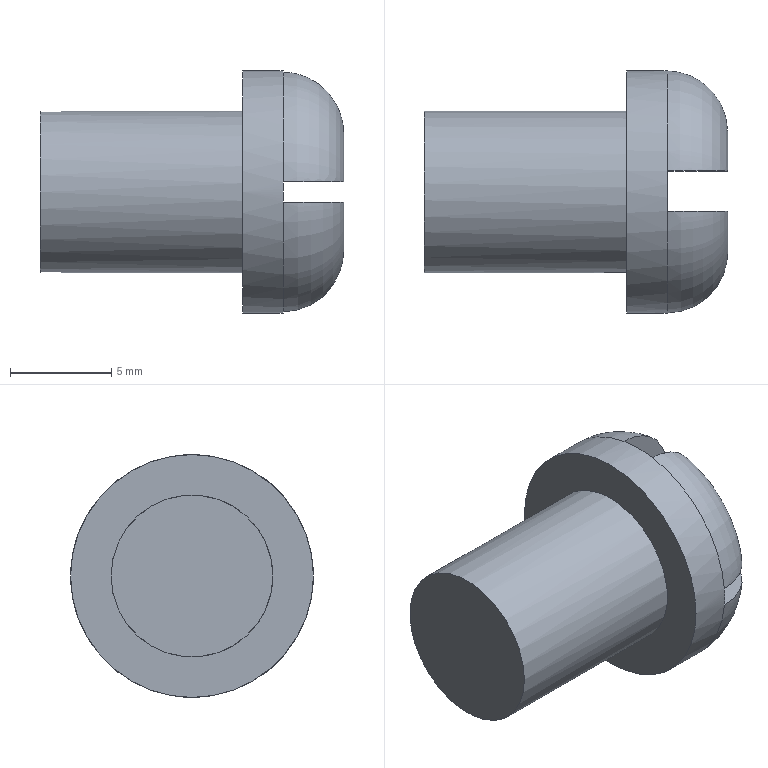Part | NX | features solid 2 | 1 solid | 25 faces | box 15 x 12 x 12 mm | volume 904.205 mm3 | plane 15 | torus 4 | sphere 4 | cylinder 2 | commonest cylinder face diameters 8 x1 12 x1
STEP:
#1=CARTESIAN_POINT('',(1114.,-196.958,-382.691));
#2=VERTEX_POINT('',#1);
#3=CARTESIAN_POINT('',(1114.,-198.449,-384.5));
#4=VERTEX_POINT('',#3);
#5=CARTESIAN_POINT('',(1114.,-196.,-385.));
#6=DIRECTION('',(-1.,0.,0.));
#7=DIRECTION('',(0.,1.,0.));
#8=AXIS2_PLACEMENT_3D('',#5,#6,#7);
#9=CIRCLE('',#8,2.5);
#10=EDGE_CURVE('',#2,#4,#9,.F.);
#11=ORIENTED_EDGE('',*,*,#10,.F.);
#12=CARTESIAN_POINT('',(1114.,-196.958,-382.157));
#13=VERTEX_POINT('',#12);
#14=CARTESIAN_POINT('',(1114.,-196.958,-385.));
#15=DIRECTION('',(0.,0.,1.));
#16=VECTOR('',#15,1000.);
#17=LINE('',#14,#16);
#18=EDGE_CURVE('',#2,#13,#17,.T.);
#19=ORIENTED_EDGE('',*,*,#18,.T.);
#20=CARTESIAN_POINT('',(1114.,-198.958,-384.5));
#21=VERTEX_POINT('',#20);
#22=CARTESIAN_POINT('',(1114.,-196.,-385.));
#23=DIRECTION('',(1.,0.,0.));
#24=DIRECTION('',(0.,-1.,0.));
#25=AXIS2_PLACEMENT_3D('',#22,#23,#24);
#26=CIRCLE('',#25,3.);
#27=EDGE_CURVE('',#13,#21,#26,.T.);
#28=ORIENTED_EDGE('',*,*,#27,.T.);
#29=CARTESIAN_POINT('',(1114.,-196.,-384.5));
#30=DIRECTION('',(0.,1.,0.));
#31=VECTOR('',#30,1000.);
#32=LINE('',#29,#31);
#33=EDGE_CURVE('',#21,#4,#32,.T.);
#34=ORIENTED_EDGE('',*,*,#33,.T.);
#35=EDGE_LOOP('',(#11,#19,#28,#34));
#36=FACE_BOUND('',#35,.T.);
#37=CARTESIAN_POINT('',(1114.,-196.,-385.));
#38=DIRECTION('',(1.,0.,0.));
#39=DIRECTION('',(0.,-1.,0.));
#40=AXIS2_PLACEMENT_3D('',#37,#38,#39);
#41=PLANE('',#40);
#42=ADVANCED_FACE('',(#36),#41,.T.);
#43=CARTESIAN_POINT('',(1111.,-201.979,-384.5));
#44=VERTEX_POINT('',#43);
#45=CARTESIAN_POINT('',(1111.,-196.958,-379.077));
#46=VERTEX_POINT('',#45);
#47=CARTESIAN_POINT('',(1111.,-196.,-385.));
#48=DIRECTION('',(1.,0.,0.));
#49=DIRECTION('',(0.,-1.,0.));
#50=AXIS2_PLACEMENT_3D('',#47,#48,#49);
#51=CIRCLE('',#50,6.);
#52=EDGE_CURVE('',#44,#46,#51,.F.);
#53=ORIENTED_EDGE('',*,*,#52,.F.);
#54=CARTESIAN_POINT('',(1111.,-201.979,-384.5));
#55=CARTESIAN_POINT('',(1111.791,-201.979,-384.5));
#56=CARTESIAN_POINT('',(1113.356,-201.32,-384.5));
#57=CARTESIAN_POINT('',(1114.,-199.752,-384.5));
#58=CARTESIAN_POINT('',(1114.,-198.958,-384.5));
#59=B_SPLINE_CURVE_WITH_KNOTS('',3,(#54,#55,#56,#57,#58),.UNSPECIFIED.,.F.,.F.,(4,1,4),(0.02837,0.03072,0.03307),.UNSPECIFIED.);
#60=EDGE_CURVE('',#44,#21,#59,.T.);
#61=ORIENTED_EDGE('',*,*,#60,.T.);
#62=ORIENTED_EDGE('',*,*,#27,.F.);
#63=CARTESIAN_POINT('',(1114.,-196.958,-382.157));
#64=CARTESIAN_POINT('',(1114.,-196.958,-381.36));
#65=CARTESIAN_POINT('',(1113.387,-196.958,-379.763));
#66=CARTESIAN_POINT('',(1111.795,-196.958,-379.077));
#67=CARTESIAN_POINT('',(1111.,-196.958,-379.077));
#68=B_SPLINE_CURVE_WITH_KNOTS('',3,(#63,#64,#65,#66,#67),.UNSPECIFIED.,.F.,.F.,(4,1,4),(0.00296,0.005334,0.007708),.UNSPECIFIED.);
#69=EDGE_CURVE('',#13,#46,#68,.T.);
#70=ORIENTED_EDGE('',*,*,#69,.T.);
#71=EDGE_LOOP('',(#53,#61,#62,#70));
#72=FACE_BOUND('',#71,.T.);
#73=CARTESIAN_POINT('',(1111.,-196.,-385.));
#74=DIRECTION('',(1.,0.,0.));
#75=DIRECTION('',(0.,-1.,0.));
#76=AXIS2_PLACEMENT_3D('',#73,#74,#75);
#77=TOROIDAL_SURFACE('',#76,3.,3.);
#78=ADVANCED_FACE('',(#72),#77,.T.);
#79=CARTESIAN_POINT('',(1114.,-193.551,-384.5));
#80=VERTEX_POINT('',#79);
#81=CARTESIAN_POINT('',(1114.,-194.958,-382.727));
#82=VERTEX_POINT('',#81);
#83=CARTESIAN_POINT('',(1114.,-196.,-385.));
#84=DIRECTION('',(-1.,0.,0.));
#85=DIRECTION('',(0.,1.,0.));
#86=AXIS2_PLACEMENT_3D('',#83,#84,#85);
#87=CIRCLE('',#86,2.5);
#88=EDGE_CURVE('',#80,#82,#87,.F.);
#89=ORIENTED_EDGE('',*,*,#88,.F.);
#90=CARTESIAN_POINT('',(1114.,-193.042,-384.5));
#91=VERTEX_POINT('',#90);
#92=CARTESIAN_POINT('',(1114.,-196.,-384.5));
#93=DIRECTION('',(0.,1.,0.));
#94=VECTOR('',#93,1000.);
#95=LINE('',#92,#94);
#96=EDGE_CURVE('',#80,#91,#95,.T.);
#97=ORIENTED_EDGE('',*,*,#96,.T.);
#98=CARTESIAN_POINT('',(1114.,-194.958,-382.187));
#99=VERTEX_POINT('',#98);
#100=CARTESIAN_POINT('',(1114.,-196.,-385.));
#101=DIRECTION('',(1.,0.,0.));
#102=DIRECTION('',(0.,-1.,0.));
#103=AXIS2_PLACEMENT_3D('',#100,#101,#102);
#104=CIRCLE('',#103,3.);
#105=EDGE_CURVE('',#91,#99,#104,.T.);
#106=ORIENTED_EDGE('',*,*,#105,.T.);
#107=CARTESIAN_POINT('',(1114.,-194.958,-385.));
#108=DIRECTION('',(0.,0.,1.));
#109=VECTOR('',#108,1000.);
#110=LINE('',#107,#109);
#111=EDGE_CURVE('',#82,#99,#110,.T.);
#112=ORIENTED_EDGE('',*,*,#111,.F.);
#113=EDGE_LOOP('',(#89,#97,#106,#112));
#114=FACE_BOUND('',#113,.T.);
#115=CARTESIAN_POINT('',(1114.,-196.,-385.));
#116=DIRECTION('',(1.,0.,0.));
#117=DIRECTION('',(0.,-1.,0.));
#118=AXIS2_PLACEMENT_3D('',#115,#116,#117);
#119=PLANE('',#118);
#120=ADVANCED_FACE('',(#114),#119,.T.);
#121=ORIENTED_EDGE('',*,*,#105,.F.);
#122=CARTESIAN_POINT('',(1111.,-190.021,-384.5));
#123=VERTEX_POINT('',#122);
#124=CARTESIAN_POINT('',(1114.,-193.042,-384.5));
#125=CARTESIAN_POINT('',(1114.,-192.251,-384.5));
#126=CARTESIAN_POINT('',(1113.359,-190.679,-384.5));
#127=CARTESIAN_POINT('',(1111.785,-190.021,-384.5));
#128=CARTESIAN_POINT('',(1111.,-190.021,-384.5));
#129=B_SPLINE_CURVE_WITH_KNOTS('',3,(#124,#125,#126,#127,#128),.UNSPECIFIED.,.F.,.F.,(4,1,4),(0.03191,0.03426,0.03662),.UNSPECIFIED.);
#130=EDGE_CURVE('',#91,#123,#129,.T.);
#131=ORIENTED_EDGE('',*,*,#130,.T.);
#132=CARTESIAN_POINT('',(1111.,-194.958,-379.091));
#133=VERTEX_POINT('',#132);
#134=CARTESIAN_POINT('',(1111.,-196.,-385.));
#135=DIRECTION('',(1.,0.,0.));
#136=DIRECTION('',(0.,-1.,0.));
#137=AXIS2_PLACEMENT_3D('',#134,#135,#136);
#138=CIRCLE('',#137,6.);
#139=EDGE_CURVE('',#133,#123,#138,.F.);
#140=ORIENTED_EDGE('',*,*,#139,.F.);
#141=CARTESIAN_POINT('',(1114.,-194.958,-382.187));
#142=CARTESIAN_POINT('',(1114.,-194.958,-381.386));
#143=CARTESIAN_POINT('',(1113.387,-194.958,-379.777));
#144=CARTESIAN_POINT('',(1111.797,-194.958,-379.091));
#145=CARTESIAN_POINT('',(1111.,-194.958,-379.091));
#146=B_SPLINE_CURVE_WITH_KNOTS('',3,(#141,#142,#143,#144,#145),.UNSPECIFIED.,.F.,.F.,(4,1,4),(0.002468,0.004872,0.007277),.UNSPECIFIED.);
#147=EDGE_CURVE('',#99,#133,#146,.T.);
#148=ORIENTED_EDGE('',*,*,#147,.F.);
#149=EDGE_LOOP('',(#121,#131,#140,#148));
#150=FACE_BOUND('',#149,.T.);
#151=CARTESIAN_POINT('',(1111.,-196.,-385.));
#152=DIRECTION('',(1.,0.,0.));
#153=DIRECTION('',(0.,-1.,0.));
#154=AXIS2_PLACEMENT_3D('',#151,#152,#153);
#155=TOROIDAL_SURFACE('',#154,3.,3.);
#156=ADVANCED_FACE('',(#150),#155,.T.);
#157=CARTESIAN_POINT('',(1111.746,-196.958,-384.5));
#158=VERTEX_POINT('',#157);
#159=CARTESIAN_POINT('',(1114.,-196.958,-385.));
#160=DIRECTION('',(0.,1.,0.));
#161=DIRECTION('',(1.,0.,0.));
#162=AXIS2_PLACEMENT_3D('',#159,#160,#161);
#163=CIRCLE('',#162,2.309);
#164=EDGE_CURVE('',#158,#2,#163,.T.);
#165=ORIENTED_EDGE('',*,*,#164,.F.);
#166=CARTESIAN_POINT('',(1111.,-196.958,-384.5));
#167=VERTEX_POINT('',#166);
#168=CARTESIAN_POINT('',(1117.,-196.958,-384.5));
#169=DIRECTION('',(-1.,0.,0.));
#170=VECTOR('',#169,1000.);
#171=LINE('',#168,#170);
#172=EDGE_CURVE('',#158,#167,#171,.T.);
#173=ORIENTED_EDGE('',*,*,#172,.T.);
#174=CARTESIAN_POINT('',(1111.,-196.958,-371.542));
#175=DIRECTION('',(0.,0.,1.));
#176=VECTOR('',#175,1000.);
#177=LINE('',#174,#176);
#178=EDGE_CURVE('',#46,#167,#177,.F.);
#179=ORIENTED_EDGE('',*,*,#178,.F.);
#180=ORIENTED_EDGE('',*,*,#69,.F.);
#181=ORIENTED_EDGE('',*,*,#18,.F.);
#182=EDGE_LOOP('',(#165,#173,#179,#180,#181));
#183=FACE_BOUND('',#182,.T.);
#184=CARTESIAN_POINT('',(1117.,-196.958,-371.542));
#185=DIRECTION('',(0.,1.,0.));
#186=DIRECTION('',(1.,0.,0.));
#187=AXIS2_PLACEMENT_3D('',#184,#185,#186);
#188=PLANE('',#187);
#189=ADVANCED_FACE('',(#183),#188,.T.);
#190=CARTESIAN_POINT('',(1111.783,-194.958,-384.5));
#191=VERTEX_POINT('',#190);
#192=CARTESIAN_POINT('',(1111.,-194.958,-384.5));
#193=VERTEX_POINT('',#192);
#194=CARTESIAN_POINT('',(1117.,-194.958,-384.5));
#195=DIRECTION('',(-1.,0.,0.));
#196=VECTOR('',#195,1000.);
#197=LINE('',#194,#196);
#198=EDGE_CURVE('',#191,#193,#197,.T.);
#199=ORIENTED_EDGE('',*,*,#198,.F.);
#200=CARTESIAN_POINT('',(1114.,-194.958,-385.));
#201=DIRECTION('',(0.,1.,0.));
#202=DIRECTION('',(1.,0.,0.));
#203=AXIS2_PLACEMENT_3D('',#200,#201,#202);
#204=CIRCLE('',#203,2.273);
#205=EDGE_CURVE('',#191,#82,#204,.T.);
#206=ORIENTED_EDGE('',*,*,#205,.T.);
#207=ORIENTED_EDGE('',*,*,#111,.T.);
#208=ORIENTED_EDGE('',*,*,#147,.T.);
#209=CARTESIAN_POINT('',(1111.,-194.958,-371.542));
#210=DIRECTION('',(0.,0.,1.));
#211=VECTOR('',#210,1000.);
#212=LINE('',#209,#211);
#213=EDGE_CURVE('',#133,#193,#212,.F.);
#214=ORIENTED_EDGE('',*,*,#213,.T.);
#215=EDGE_LOOP('',(#199,#206,#207,#208,#214));
#216=FACE_BOUND('',#215,.T.);
#217=CARTESIAN_POINT('',(1117.,-194.958,-371.542));
#218=DIRECTION('',(0.,1.,0.));
#219=DIRECTION('',(1.,0.,0.));
#220=AXIS2_PLACEMENT_3D('',#217,#218,#219);
#221=PLANE('',#220);
#222=ADVANCED_FACE('',(#216),#221,.F.);
#223=CARTESIAN_POINT('',(1114.,-198.449,-385.5));
#224=VERTEX_POINT('',#223);
#225=CARTESIAN_POINT('',(1114.,-196.958,-387.309));
#226=VERTEX_POINT('',#225);
#227=CARTESIAN_POINT('',(1114.,-196.,-385.));
#228=DIRECTION('',(-1.,0.,0.));
#229=DIRECTION('',(0.,1.,0.));
#230=AXIS2_PLACEMENT_3D('',#227,#228,#229);
#231=CIRCLE('',#230,2.5);
#232=EDGE_CURVE('',#224,#226,#231,.F.);
#233=ORIENTED_EDGE('',*,*,#232,.F.);
#234=CARTESIAN_POINT('',(1114.,-198.958,-385.5));
#235=VERTEX_POINT('',#234);
#236=CARTESIAN_POINT('',(1114.,-196.,-385.5));
#237=DIRECTION('',(0.,1.,0.));
#238=VECTOR('',#237,1000.);
#239=LINE('',#236,#238);
#240=EDGE_CURVE('',#235,#224,#239,.T.);
#241=ORIENTED_EDGE('',*,*,#240,.F.);
#242=CARTESIAN_POINT('',(1114.,-196.958,-387.843));
#243=VERTEX_POINT('',#242);
#244=CARTESIAN_POINT('',(1114.,-196.,-385.));
#245=DIRECTION('',(1.,0.,0.));
#246=DIRECTION('',(0.,-1.,0.));
#247=AXIS2_PLACEMENT_3D('',#244,#245,#246);
#248=CIRCLE('',#247,3.);
#249=EDGE_CURVE('',#235,#243,#248,.T.);
#250=ORIENTED_EDGE('',*,*,#249,.T.);
#251=CARTESIAN_POINT('',(1114.,-196.958,-385.));
#252=DIRECTION('',(0.,0.,1.));
#253=VECTOR('',#252,1000.);
#254=LINE('',#251,#253);
#255=EDGE_CURVE('',#243,#226,#254,.T.);
#256=ORIENTED_EDGE('',*,*,#255,.T.);
#257=EDGE_LOOP('',(#233,#241,#250,#256));
#258=FACE_BOUND('',#257,.T.);
#259=CARTESIAN_POINT('',(1114.,-196.,-385.));
#260=DIRECTION('',(1.,0.,0.));
#261=DIRECTION('',(0.,-1.,0.));
#262=AXIS2_PLACEMENT_3D('',#259,#260,#261);
#263=PLANE('',#262);
#264=ADVANCED_FACE('',(#258),#263,.T.);
#265=CARTESIAN_POINT('',(1111.,-201.979,-385.5));
#266=VERTEX_POINT('',#265);
#267=CARTESIAN_POINT('',(1111.,-201.979,-385.5));
#268=CARTESIAN_POINT('',(1111.791,-201.979,-385.5));
#269=CARTESIAN_POINT('',(1113.356,-201.32,-385.5));
#270=CARTESIAN_POINT('',(1114.,-199.752,-385.5));
#271=CARTESIAN_POINT('',(1114.,-198.958,-385.5));
#272=B_SPLINE_CURVE_WITH_KNOTS('',3,(#267,#268,#269,#270,#271),.UNSPECIFIED.,.F.,.F.,(4,1,4),(0.02837,0.03072,0.03307),.UNSPECIFIED.);
#273=EDGE_CURVE('',#266,#235,#272,.T.);
#274=ORIENTED_EDGE('',*,*,#273,.F.);
#275=CARTESIAN_POINT('',(1111.,-196.958,-390.923));
#276=VERTEX_POINT('',#275);
#277=CARTESIAN_POINT('',(1111.,-196.,-385.));
#278=DIRECTION('',(1.,0.,0.));
#279=DIRECTION('',(0.,-1.,0.));
#280=AXIS2_PLACEMENT_3D('',#277,#278,#279);
#281=CIRCLE('',#280,6.);
#282=EDGE_CURVE('',#276,#266,#281,.F.);
#283=ORIENTED_EDGE('',*,*,#282,.F.);
#284=CARTESIAN_POINT('',(1111.,-196.958,-390.923));
#285=CARTESIAN_POINT('',(1111.798,-196.958,-390.923));
#286=CARTESIAN_POINT('',(1113.382,-196.958,-390.24));
#287=CARTESIAN_POINT('',(1114.,-196.958,-388.644));
#288=CARTESIAN_POINT('',(1114.,-196.958,-387.843));
#289=B_SPLINE_CURVE_WITH_KNOTS('',3,(#284,#285,#286,#287,#288),.UNSPECIFIED.,.F.,.F.,(4,1,4),(0.02303,0.02538,0.02772),.UNSPECIFIED.);
#290=EDGE_CURVE('',#276,#243,#289,.T.);
#291=ORIENTED_EDGE('',*,*,#290,.T.);
#292=ORIENTED_EDGE('',*,*,#249,.F.);
#293=EDGE_LOOP('',(#274,#283,#291,#292));
#294=FACE_BOUND('',#293,.T.);
#295=CARTESIAN_POINT('',(1111.,-196.,-385.));
#296=DIRECTION('',(1.,0.,0.));
#297=DIRECTION('',(0.,-1.,0.));
#298=AXIS2_PLACEMENT_3D('',#295,#296,#297);
#299=TOROIDAL_SURFACE('',#298,3.,3.);
#300=ADVANCED_FACE('',(#294),#299,.T.);
#301=CARTESIAN_POINT('',(1114.,-194.958,-387.273));
#302=VERTEX_POINT('',#301);
#303=CARTESIAN_POINT('',(1114.,-193.551,-385.5));
#304=VERTEX_POINT('',#303);
#305=CARTESIAN_POINT('',(1114.,-196.,-385.));
#306=DIRECTION('',(-1.,0.,0.));
#307=DIRECTION('',(0.,1.,0.));
#308=AXIS2_PLACEMENT_3D('',#305,#306,#307);
#309=CIRCLE('',#308,2.5);
#310=EDGE_CURVE('',#302,#304,#309,.F.);
#311=ORIENTED_EDGE('',*,*,#310,.F.);
#312=CARTESIAN_POINT('',(1114.,-194.958,-387.813));
#313=VERTEX_POINT('',#312);
#314=CARTESIAN_POINT('',(1114.,-194.958,-385.));
#315=DIRECTION('',(0.,0.,1.));
#316=VECTOR('',#315,1000.);
#317=LINE('',#314,#316);
#318=EDGE_CURVE('',#313,#302,#317,.T.);
#319=ORIENTED_EDGE('',*,*,#318,.F.);
#320=CARTESIAN_POINT('',(1114.,-193.042,-385.5));
#321=VERTEX_POINT('',#320);
#322=CARTESIAN_POINT('',(1114.,-196.,-385.));
#323=DIRECTION('',(1.,0.,0.));
#324=DIRECTION('',(0.,-1.,0.));
#325=AXIS2_PLACEMENT_3D('',#322,#323,#324);
#326=CIRCLE('',#325,3.);
#327=EDGE_CURVE('',#313,#321,#326,.T.);
#328=ORIENTED_EDGE('',*,*,#327,.T.);
#329=CARTESIAN_POINT('',(1114.,-196.,-385.5));
#330=DIRECTION('',(0.,1.,0.));
#331=VECTOR('',#330,1000.);
#332=LINE('',#329,#331);
#333=EDGE_CURVE('',#304,#321,#332,.T.);
#334=ORIENTED_EDGE('',*,*,#333,.F.);
#335=EDGE_LOOP('',(#311,#319,#328,#334));
#336=FACE_BOUND('',#335,.T.);
#337=CARTESIAN_POINT('',(1114.,-196.,-385.));
#338=DIRECTION('',(1.,0.,0.));
#339=DIRECTION('',(0.,-1.,0.));
#340=AXIS2_PLACEMENT_3D('',#337,#338,#339);
#341=PLANE('',#340);
#342=ADVANCED_FACE('',(#336),#341,.T.);
#343=CARTESIAN_POINT('',(1109.,-192.,-385.));
#344=VERTEX_POINT('',#343);
#345=CARTESIAN_POINT('',(1109.,-196.,-385.));
#346=DIRECTION('',(-1.,0.,0.));
#347=DIRECTION('',(0.,1.,0.));
#348=AXIS2_PLACEMENT_3D('',#345,#346,#347);
#349=CIRCLE('',#348,4.);
#350=EDGE_CURVE('',#344,#344,#349,.T.);
#351=ORIENTED_EDGE('',*,*,#350,.F.);
#352=EDGE_LOOP('',(#351));
#353=FACE_BOUND('',#352,.T.);
#354=CARTESIAN_POINT('',(1109.,-202.,-385.));
#355=VERTEX_POINT('',#354);
#356=CARTESIAN_POINT('',(1109.,-196.,-385.));
#357=DIRECTION('',(1.,0.,0.));
#358=DIRECTION('',(0.,-1.,0.));
#359=AXIS2_PLACEMENT_3D('',#356,#357,#358);
#360=CIRCLE('',#359,6.);
#361=EDGE_CURVE('',#355,#355,#360,.T.);
#362=ORIENTED_EDGE('',*,*,#361,.F.);
#363=EDGE_LOOP('',(#362));
#364=FACE_BOUND('',#363,.T.);
#365=CARTESIAN_POINT('',(1109.,-196.,-385.));
#366=DIRECTION('',(-1.,0.,0.));
#367=DIRECTION('',(0.,1.,0.));
#368=AXIS2_PLACEMENT_3D('',#365,#366,#367);
#369=PLANE('',#368);
#370=ADVANCED_FACE('',(#353,#364),#369,.T.);
#371=CARTESIAN_POINT('',(1111.,-196.,-385.));
#372=DIRECTION('',(1.,0.,0.));
#373=DIRECTION('',(0.,-1.,0.));
#374=AXIS2_PLACEMENT_3D('',#371,#372,#373);
#375=CIRCLE('',#374,6.);
#376=EDGE_CURVE('',#133,#46,#375,.T.);
#377=ORIENTED_EDGE('',*,*,#376,.F.);
#378=ORIENTED_EDGE('',*,*,#139,.T.);
#379=CARTESIAN_POINT('',(1111.,-190.021,-385.5));
#380=VERTEX_POINT('',#379);
#381=CARTESIAN_POINT('',(1111.,-196.,-385.));
#382=DIRECTION('',(1.,0.,0.));
#383=DIRECTION('',(0.,-1.,0.));
#384=AXIS2_PLACEMENT_3D('',#381,#382,#383);
#385=CIRCLE('',#384,6.);
#386=EDGE_CURVE('',#380,#123,#385,.T.);
#387=ORIENTED_EDGE('',*,*,#386,.F.);
#388=CARTESIAN_POINT('',(1111.,-194.958,-390.909));
#389=VERTEX_POINT('',#388);
#390=CARTESIAN_POINT('',(1111.,-196.,-385.));
#391=DIRECTION('',(1.,0.,0.));
#392=DIRECTION('',(0.,-1.,0.));
#393=AXIS2_PLACEMENT_3D('',#390,#391,#392);
#394=CIRCLE('',#393,6.);
#395=EDGE_CURVE('',#380,#389,#394,.F.);
#396=ORIENTED_EDGE('',*,*,#395,.T.);
#397=CARTESIAN_POINT('',(1111.,-196.,-385.));
#398=DIRECTION('',(1.,0.,0.));
#399=DIRECTION('',(0.,-1.,0.));
#400=AXIS2_PLACEMENT_3D('',#397,#398,#399);
#401=CIRCLE('',#400,6.);
#402=EDGE_CURVE('',#276,#389,#401,.T.);
#403=ORIENTED_EDGE('',*,*,#402,.F.);
#404=ORIENTED_EDGE('',*,*,#282,.T.);
#405=CARTESIAN_POINT('',(1111.,-196.,-385.));
#406=DIRECTION('',(1.,0.,0.));
#407=DIRECTION('',(0.,-1.,0.));
#408=AXIS2_PLACEMENT_3D('',#405,#406,#407);
#409=CIRCLE('',#408,6.);
#410=EDGE_CURVE('',#44,#266,#409,.T.);
#411=ORIENTED_EDGE('',*,*,#410,.F.);
#412=ORIENTED_EDGE('',*,*,#52,.T.);
#413=EDGE_LOOP('',(#377,#378,#387,#396,#403,#404,#411,#412));
#414=FACE_BOUND('',#413,.T.);
#415=ORIENTED_EDGE('',*,*,#361,.T.);
#416=EDGE_LOOP('',(#415));
#417=FACE_BOUND('',#416,.T.);
#418=CARTESIAN_POINT('',(1109.,-196.,-385.));
#419=DIRECTION('',(1.,0.,0.));
#420=DIRECTION('',(0.,-1.,0.));
#421=AXIS2_PLACEMENT_3D('',#418,#419,#420);
#422=CYLINDRICAL_SURFACE('',#421,6.);
#423=ADVANCED_FACE('',(#414,#417),#422,.T.);
#424=CARTESIAN_POINT('',(1099.,-200.,-385.));
#425=VERTEX_POINT('',#424);
#426=CARTESIAN_POINT('',(1099.,-196.,-385.));
#427=DIRECTION('',(1.,0.,0.));
#428=DIRECTION('',(0.,-1.,0.));
#429=AXIS2_PLACEMENT_3D('',#426,#427,#428);
#430=CIRCLE('',#429,4.);
#431=EDGE_CURVE('',#425,#425,#430,.T.);
#432=ORIENTED_EDGE('',*,*,#431,.F.);
#433=EDGE_LOOP('',(#432));
#434=FACE_BOUND('',#433,.T.);
#435=CARTESIAN_POINT('',(1099.,-196.,-385.));
#436=DIRECTION('',(-1.,0.,0.));
#437=DIRECTION('',(0.,1.,0.));
#438=AXIS2_PLACEMENT_3D('',#435,#436,#437);
#439=PLANE('',#438);
#440=ADVANCED_FACE('',(#434),#439,.T.);
#441=ORIENTED_EDGE('',*,*,#431,.T.);
#442=EDGE_LOOP('',(#441));
#443=FACE_BOUND('',#442,.T.);
#444=ORIENTED_EDGE('',*,*,#350,.T.);
#445=EDGE_LOOP('',(#444));
#446=FACE_BOUND('',#445,.T.);
#447=CARTESIAN_POINT('',(1109.,-196.,-385.));
#448=DIRECTION('',(-1.,0.,0.));
#449=DIRECTION('',(0.,1.,0.));
#450=AXIS2_PLACEMENT_3D('',#447,#448,#449);
#451=CYLINDRICAL_SURFACE('',#450,4.);
#452=ADVANCED_FACE('',(#443,#446),#451,.T.);
#453=CARTESIAN_POINT('',(1114.,-193.042,-385.5));
#454=CARTESIAN_POINT('',(1114.,-192.251,-385.5));
#455=CARTESIAN_POINT('',(1113.359,-190.679,-385.5));
#456=CARTESIAN_POINT('',(1111.785,-190.021,-385.5));
#457=CARTESIAN_POINT('',(1111.,-190.021,-385.5));
#458=B_SPLINE_CURVE_WITH_KNOTS('',3,(#453,#454,#455,#456,#457),.UNSPECIFIED.,.F.,.F.,(4,1,4),(0.03191,0.03426,0.03662),.UNSPECIFIED.);
#459=EDGE_CURVE('',#321,#380,#458,.T.);
#460=ORIENTED_EDGE('',*,*,#459,.F.);
#461=ORIENTED_EDGE('',*,*,#327,.F.);
#462=CARTESIAN_POINT('',(1114.,-194.958,-387.813));
#463=CARTESIAN_POINT('',(1114.,-194.958,-388.611));
#464=CARTESIAN_POINT('',(1113.39,-194.958,-390.222));
#465=CARTESIAN_POINT('',(1111.796,-194.958,-390.909));
#466=CARTESIAN_POINT('',(1111.,-194.958,-390.909));
#467=B_SPLINE_CURVE_WITH_KNOTS('',3,(#462,#463,#464,#465,#466),.UNSPECIFIED.,.F.,.F.,(4,1,4),(0.009658,0.01206,0.01445),.UNSPECIFIED.);
#468=EDGE_CURVE('',#389,#313,#467,.F.);
#469=ORIENTED_EDGE('',*,*,#468,.F.);
#470=ORIENTED_EDGE('',*,*,#395,.F.);
#471=EDGE_LOOP('',(#460,#461,#469,#470));
#472=FACE_BOUND('',#471,.T.);
#473=CARTESIAN_POINT('',(1111.,-196.,-385.));
#474=DIRECTION('',(1.,0.,0.));
#475=DIRECTION('',(0.,-1.,0.));
#476=AXIS2_PLACEMENT_3D('',#473,#474,#475);
#477=TOROIDAL_SURFACE('',#476,3.,3.);
#478=ADVANCED_FACE('',(#472),#477,.T.);
#479=CARTESIAN_POINT('',(1111.,-194.958,-385.5));
#480=VERTEX_POINT('',#479);
#481=CARTESIAN_POINT('',(1111.,-194.958,-371.542));
#482=DIRECTION('',(0.,0.,1.));
#483=VECTOR('',#482,1000.);
#484=LINE('',#481,#483);
#485=EDGE_CURVE('',#480,#389,#484,.F.);
#486=ORIENTED_EDGE('',*,*,#485,.F.);
#487=CARTESIAN_POINT('',(1111.,-101.,-385.5));
#488=DIRECTION('',(0.,1.,0.));
#489=VECTOR('',#488,1000.);
#490=LINE('',#487,#489);
#491=EDGE_CURVE('',#380,#480,#490,.F.);
#492=ORIENTED_EDGE('',*,*,#491,.F.);
#493=ORIENTED_EDGE('',*,*,#386,.T.);
#494=CARTESIAN_POINT('',(1111.,-101.,-384.5));
#495=DIRECTION('',(0.,1.,0.));
#496=VECTOR('',#495,1000.);
#497=LINE('',#494,#496);
#498=EDGE_CURVE('',#123,#193,#497,.F.);
#499=ORIENTED_EDGE('',*,*,#498,.T.);
#500=ORIENTED_EDGE('',*,*,#213,.F.);
#501=ORIENTED_EDGE('',*,*,#376,.T.);
#502=ORIENTED_EDGE('',*,*,#178,.T.);
#503=CARTESIAN_POINT('',(1111.,-101.,-384.5));
#504=DIRECTION('',(0.,1.,0.));
#505=VECTOR('',#504,1000.);
#506=LINE('',#503,#505);
#507=EDGE_CURVE('',#167,#44,#506,.F.);
#508=ORIENTED_EDGE('',*,*,#507,.T.);
#509=ORIENTED_EDGE('',*,*,#410,.T.);
#510=CARTESIAN_POINT('',(1111.,-196.958,-385.5));
#511=VERTEX_POINT('',#510);
#512=CARTESIAN_POINT('',(1111.,-101.,-385.5));
#513=DIRECTION('',(0.,1.,0.));
#514=VECTOR('',#513,1000.);
#515=LINE('',#512,#514);
#516=EDGE_CURVE('',#511,#266,#515,.F.);
#517=ORIENTED_EDGE('',*,*,#516,.F.);
#518=CARTESIAN_POINT('',(1111.,-196.958,-371.542));
#519=DIRECTION('',(0.,0.,1.));
#520=VECTOR('',#519,1000.);
#521=LINE('',#518,#520);
#522=EDGE_CURVE('',#511,#276,#521,.F.);
#523=ORIENTED_EDGE('',*,*,#522,.T.);
#524=ORIENTED_EDGE('',*,*,#402,.T.);
#525=EDGE_LOOP('',(#486,#492,#493,#499,#500,#501,#502,#508,#509,#517,#523,#524));
#526=FACE_BOUND('',#525,.T.);
#527=CARTESIAN_POINT('',(1111.,-196.458,-371.542));
#528=DIRECTION('',(1.,0.,0.));
#529=DIRECTION('',(0.,0.,-1.));
#530=AXIS2_PLACEMENT_3D('',#527,#528,#529);
#531=PLANE('',#530);
#532=ADVANCED_FACE('',(#526),#531,.T.);
#533=CARTESIAN_POINT('',(1111.746,-196.958,-385.5));
#534=VERTEX_POINT('',#533);
#535=CARTESIAN_POINT('',(1114.,-196.958,-385.));
#536=DIRECTION('',(0.,1.,0.));
#537=DIRECTION('',(1.,0.,0.));
#538=AXIS2_PLACEMENT_3D('',#535,#536,#537);
#539=CIRCLE('',#538,2.309);
#540=EDGE_CURVE('',#226,#534,#539,.T.);
#541=ORIENTED_EDGE('',*,*,#540,.F.);
#542=ORIENTED_EDGE('',*,*,#255,.F.);
#543=ORIENTED_EDGE('',*,*,#290,.F.);
#544=ORIENTED_EDGE('',*,*,#522,.F.);
#545=CARTESIAN_POINT('',(1117.,-196.958,-385.5));
#546=DIRECTION('',(-1.,0.,0.));
#547=VECTOR('',#546,1000.);
#548=LINE('',#545,#547);
#549=EDGE_CURVE('',#534,#511,#548,.T.);
#550=ORIENTED_EDGE('',*,*,#549,.F.);
#551=EDGE_LOOP('',(#541,#542,#543,#544,#550));
#552=FACE_BOUND('',#551,.T.);
#553=CARTESIAN_POINT('',(1117.,-196.958,-371.542));
#554=DIRECTION('',(0.,1.,0.));
#555=DIRECTION('',(1.,0.,0.));
#556=AXIS2_PLACEMENT_3D('',#553,#554,#555);
#557=PLANE('',#556);
#558=ADVANCED_FACE('',(#552),#557,.T.);
#559=ORIENTED_EDGE('',*,*,#318,.T.);
#560=CARTESIAN_POINT('',(1111.783,-194.958,-385.5));
#561=VERTEX_POINT('',#560);
#562=CARTESIAN_POINT('',(1114.,-194.958,-385.));
#563=DIRECTION('',(0.,1.,0.));
#564=DIRECTION('',(1.,0.,0.));
#565=AXIS2_PLACEMENT_3D('',#562,#563,#564);
#566=CIRCLE('',#565,2.273);
#567=EDGE_CURVE('',#302,#561,#566,.T.);
#568=ORIENTED_EDGE('',*,*,#567,.T.);
#569=CARTESIAN_POINT('',(1117.,-194.958,-385.5));
#570=DIRECTION('',(-1.,0.,0.));
#571=VECTOR('',#570,1000.);
#572=LINE('',#569,#571);
#573=EDGE_CURVE('',#561,#480,#572,.T.);
#574=ORIENTED_EDGE('',*,*,#573,.T.);
#575=ORIENTED_EDGE('',*,*,#485,.T.);
#576=ORIENTED_EDGE('',*,*,#468,.T.);
#577=EDGE_LOOP('',(#559,#568,#574,#575,#576));
#578=FACE_BOUND('',#577,.T.);
#579=CARTESIAN_POINT('',(1117.,-194.958,-371.542));
#580=DIRECTION('',(0.,1.,0.));
#581=DIRECTION('',(1.,0.,0.));
#582=AXIS2_PLACEMENT_3D('',#579,#580,#581);
#583=PLANE('',#582);
#584=ADVANCED_FACE('',(#578),#583,.F.);
#585=CARTESIAN_POINT('',(1114.,-196.,-384.5));
#586=DIRECTION('',(0.,0.,-1.));
#587=DIRECTION('',(1.,0.,0.));
#588=AXIS2_PLACEMENT_3D('',#585,#586,#587);
#589=CIRCLE('',#588,2.449);
#590=EDGE_CURVE('',#191,#80,#589,.T.);
#591=ORIENTED_EDGE('',*,*,#590,.F.);
#592=ORIENTED_EDGE('',*,*,#198,.T.);
#593=ORIENTED_EDGE('',*,*,#498,.F.);
#594=ORIENTED_EDGE('',*,*,#130,.F.);
#595=ORIENTED_EDGE('',*,*,#96,.F.);
#596=EDGE_LOOP('',(#591,#592,#593,#594,#595));
#597=FACE_BOUND('',#596,.T.);
#598=CARTESIAN_POINT('',(1117.,-101.,-384.5));
#599=DIRECTION('',(0.,0.,-1.));
#600=DIRECTION('',(1.,0.,0.));
#601=AXIS2_PLACEMENT_3D('',#598,#599,#600);
#602=PLANE('',#601);
#603=ADVANCED_FACE('',(#597),#602,.T.);
#604=ORIENTED_EDGE('',*,*,#573,.F.);
#605=CARTESIAN_POINT('',(1114.,-196.,-385.5));
#606=DIRECTION('',(0.,0.,-1.));
#607=DIRECTION('',(1.,0.,0.));
#608=AXIS2_PLACEMENT_3D('',#605,#606,#607);
#609=CIRCLE('',#608,2.449);
#610=EDGE_CURVE('',#561,#304,#609,.T.);
#611=ORIENTED_EDGE('',*,*,#610,.T.);
#612=ORIENTED_EDGE('',*,*,#333,.T.);
#613=ORIENTED_EDGE('',*,*,#459,.T.);
#614=ORIENTED_EDGE('',*,*,#491,.T.);
#615=EDGE_LOOP('',(#604,#611,#612,#613,#614));
#616=FACE_BOUND('',#615,.T.);
#617=CARTESIAN_POINT('',(1117.,-101.,-385.5));
#618=DIRECTION('',(0.,0.,-1.));
#619=DIRECTION('',(1.,0.,0.));
#620=AXIS2_PLACEMENT_3D('',#617,#618,#619);
#621=PLANE('',#620);
#622=ADVANCED_FACE('',(#616),#621,.F.);
#623=CARTESIAN_POINT('',(1114.,-196.,-384.5));
#624=DIRECTION('',(0.,0.,-1.));
#625=DIRECTION('',(1.,0.,0.));
#626=AXIS2_PLACEMENT_3D('',#623,#624,#625);
#627=CIRCLE('',#626,2.449);
#628=EDGE_CURVE('',#4,#158,#627,.T.);
#629=ORIENTED_EDGE('',*,*,#628,.F.);
#630=ORIENTED_EDGE('',*,*,#33,.F.);
#631=ORIENTED_EDGE('',*,*,#60,.F.);
#632=ORIENTED_EDGE('',*,*,#507,.F.);
#633=ORIENTED_EDGE('',*,*,#172,.F.);
#634=EDGE_LOOP('',(#629,#630,#631,#632,#633));
#635=FACE_BOUND('',#634,.T.);
#636=CARTESIAN_POINT('',(1117.,-101.,-384.5));
#637=DIRECTION('',(0.,0.,-1.));
#638=DIRECTION('',(1.,0.,0.));
#639=AXIS2_PLACEMENT_3D('',#636,#637,#638);
#640=PLANE('',#639);
#641=ADVANCED_FACE('',(#635),#640,.T.);
#642=ORIENTED_EDGE('',*,*,#240,.T.);
#643=CARTESIAN_POINT('',(1114.,-196.,-385.5));
#644=DIRECTION('',(0.,0.,-1.));
#645=DIRECTION('',(1.,0.,0.));
#646=AXIS2_PLACEMENT_3D('',#643,#644,#645);
#647=CIRCLE('',#646,2.449);
#648=EDGE_CURVE('',#224,#534,#647,.T.);
#649=ORIENTED_EDGE('',*,*,#648,.T.);
#650=ORIENTED_EDGE('',*,*,#549,.T.);
#651=ORIENTED_EDGE('',*,*,#516,.T.);
#652=ORIENTED_EDGE('',*,*,#273,.T.);
#653=EDGE_LOOP('',(#642,#649,#650,#651,#652));
#654=FACE_BOUND('',#653,.T.);
#655=CARTESIAN_POINT('',(1117.,-101.,-385.5));
#656=DIRECTION('',(0.,0.,-1.));
#657=DIRECTION('',(1.,0.,0.));
#658=AXIS2_PLACEMENT_3D('',#655,#656,#657);
#659=PLANE('',#658);
#660=ADVANCED_FACE('',(#654),#659,.F.);
#661=ORIENTED_EDGE('',*,*,#540,.T.);
#662=ORIENTED_EDGE('',*,*,#648,.F.);
#663=ORIENTED_EDGE('',*,*,#232,.T.);
#664=EDGE_LOOP('',(#661,#662,#663));
#665=FACE_BOUND('',#664,.T.);
#666=CARTESIAN_POINT('',(1114.,-196.,-385.));
#667=DIRECTION('',(1.,0.,0.));
#668=DIRECTION('',(0.,-1.,0.));
#669=AXIS2_PLACEMENT_3D('',#666,#667,#668);
#670=SPHERICAL_SURFACE('',#669,2.5);
#671=ADVANCED_FACE('',(#665),#670,.F.);
#672=ORIENTED_EDGE('',*,*,#164,.T.);
#673=ORIENTED_EDGE('',*,*,#10,.T.);
#674=ORIENTED_EDGE('',*,*,#628,.T.);
#675=EDGE_LOOP('',(#672,#673,#674));
#676=FACE_BOUND('',#675,.T.);
#677=CARTESIAN_POINT('',(1114.,-196.,-385.));
#678=DIRECTION('',(1.,0.,0.));
#679=DIRECTION('',(0.,-1.,0.));
#680=AXIS2_PLACEMENT_3D('',#677,#678,#679);
#681=SPHERICAL_SURFACE('',#680,2.5);
#682=ADVANCED_FACE('',(#676),#681,.F.);
#683=ORIENTED_EDGE('',*,*,#310,.T.);
#684=ORIENTED_EDGE('',*,*,#610,.F.);
#685=ORIENTED_EDGE('',*,*,#567,.F.);
#686=EDGE_LOOP('',(#683,#684,#685));
#687=FACE_BOUND('',#686,.T.);
#688=CARTESIAN_POINT('',(1114.,-196.,-385.));
#689=DIRECTION('',(1.,0.,0.));
#690=DIRECTION('',(0.,-1.,0.));
#691=AXIS2_PLACEMENT_3D('',#688,#689,#690);
#692=SPHERICAL_SURFACE('',#691,2.5);
#693=ADVANCED_FACE('',(#687),#692,.F.);
#694=ORIENTED_EDGE('',*,*,#590,.T.);
#695=ORIENTED_EDGE('',*,*,#88,.T.);
#696=ORIENTED_EDGE('',*,*,#205,.F.);
#697=EDGE_LOOP('',(#694,#695,#696));
#698=FACE_BOUND('',#697,.T.);
#699=CARTESIAN_POINT('',(1114.,-196.,-385.));
#700=DIRECTION('',(1.,0.,0.));
#701=DIRECTION('',(0.,-1.,0.));
#702=AXIS2_PLACEMENT_3D('',#699,#700,#701);
#703=SPHERICAL_SURFACE('',#702,2.5);
#704=ADVANCED_FACE('',(#698),#703,.F.);
#705=CLOSED_SHELL('',(#42,#78,#120,#156,#189,#222,#264,#300,#342,#370,#423,#440,#452,#478,#532,#558,#584,#603,#622,#641,#660,#671,#682,#693,#704));
#706=MANIFOLD_SOLID_BREP('',#705);
#707=(LENGTH_UNIT()NAMED_UNIT(*)SI_UNIT(.MILLI.,.METRE.));
#708=UNCERTAINTY_MEASURE_WITH_UNIT(LENGTH_MEASURE(0.0508),#707,'','');
#709=(NAMED_UNIT(*)PLANE_ANGLE_UNIT()SI_UNIT($,.RADIAN.));
#710=(NAMED_UNIT(*)SI_UNIT($,.STERADIAN.)SOLID_ANGLE_UNIT());
#711=(GEOMETRIC_REPRESENTATION_CONTEXT(3)GLOBAL_UNCERTAINTY_ASSIGNED_CONTEXT((#708))GLOBAL_UNIT_ASSIGNED_CONTEXT((#707,#709,#710))REPRESENTATION_CONTEXT('',''));
#712=ADVANCED_BREP_SHAPE_REPRESENTATION('',(#706),#711);